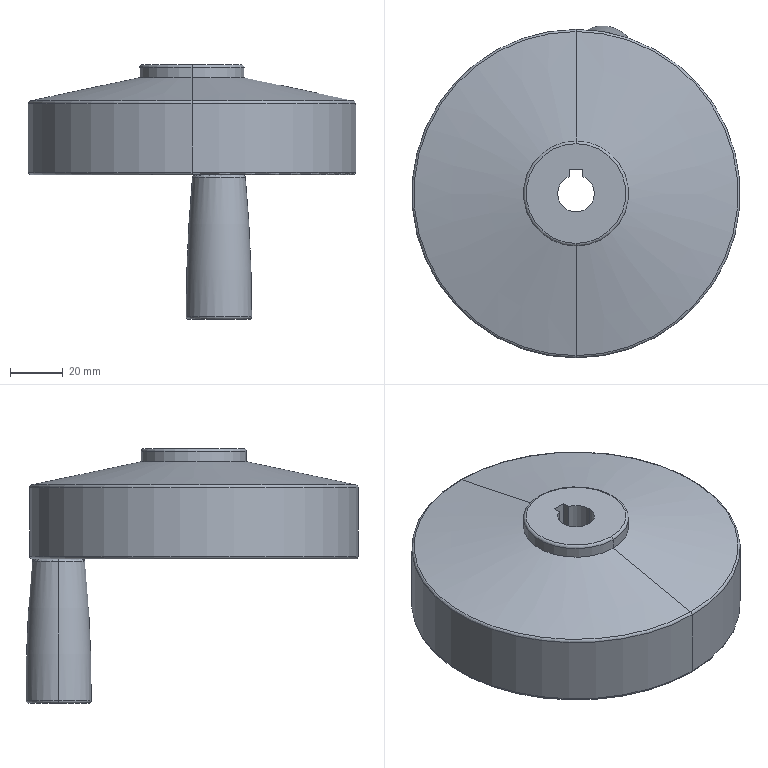Part | SolidWorks | features BaseBody 1 | 1 solid | 83 faces | box 125 x 126.49 x 97 mm | volume 263247 mm3 | cylinder 40 | plane 19 | torus 16 | cone 8 | commonest cylinder face diameters 10 x20 20 x11 14 x3 8.5 x2 40 x2 125 x2